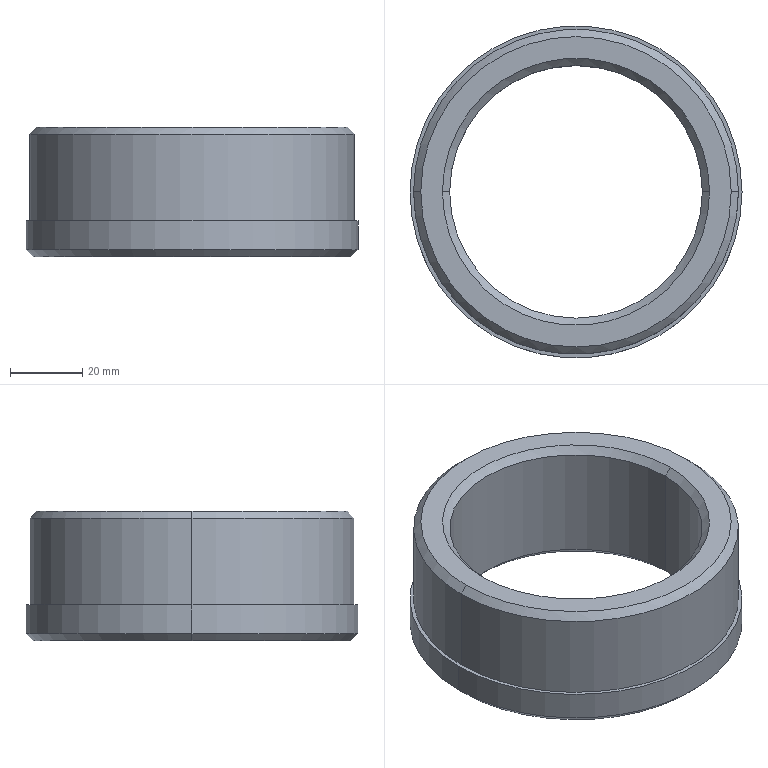Part | SolidWorks | features Chamfer 1, Revolution 1 | 1 solid | 17 faces | box 92 x 92 x 36 mm | volume 91314 mm3 | cone 8 | cylinder 6 | plane 3 | commonest cylinder face diameters 70 x2 90 x2 92 x2
STEP:
#1=CARTESIAN_POINT('',(43.,0.,0.));
#2=VERTEX_POINT('',#1);
#3=CARTESIAN_POINT('',(-43.,0.,0.));
#4=VERTEX_POINT('',#3);
#5=CARTESIAN_POINT('',(0.,0.,0.));
#6=DIRECTION('',(0.,0.,1.));
#7=DIRECTION('',(1.,0.,0.));
#8=AXIS2_PLACEMENT_3D('',#5,#6,#7);
#9=CIRCLE('',#8,43.);
#10=EDGE_CURVE('',#2,#4,#9,.T.);
#11=ORIENTED_EDGE('',*,*,#10,.F.);
#12=CARTESIAN_POINT('',(45.,0.,-2.));
#13=VERTEX_POINT('',#12);
#14=CARTESIAN_POINT('',(43.,0.,0.));
#15=DIRECTION('',(0.7071,0.,-0.7071));
#16=VECTOR('',#15,1000.);
#17=LINE('',#14,#16);
#18=EDGE_CURVE('',#2,#13,#17,.T.);
#19=ORIENTED_EDGE('',*,*,#18,.T.);
#20=CARTESIAN_POINT('',(-45.,0.,-2.));
#21=VERTEX_POINT('',#20);
#22=CARTESIAN_POINT('',(0.,0.,-2.));
#23=DIRECTION('',(0.,0.,-1.));
#24=DIRECTION('',(1.,0.,0.));
#25=AXIS2_PLACEMENT_3D('',#22,#23,#24);
#26=CIRCLE('',#25,45.);
#27=EDGE_CURVE('',#21,#13,#26,.T.);
#28=ORIENTED_EDGE('',*,*,#27,.F.);
#29=CARTESIAN_POINT('',(-43.,0.,0.));
#30=DIRECTION('',(-0.7071,0.,-0.7071));
#31=VECTOR('',#30,1000.);
#32=LINE('',#29,#31);
#33=EDGE_CURVE('',#4,#21,#32,.T.);
#34=ORIENTED_EDGE('',*,*,#33,.F.);
#35=EDGE_LOOP('',(#11,#19,#28,#34));
#36=FACE_OUTER_BOUND('',#35,.T.);
#37=CARTESIAN_POINT('',(0.,0.,0.));
#38=DIRECTION('',(0.,0.,-1.));
#39=DIRECTION('',(-1.,0.,0.));
#40=AXIS2_PLACEMENT_3D('',#37,#38,#39);
#41=CONICAL_SURFACE('',#40,43.,0.7854);
#42=ADVANCED_FACE('',(#36),#41,.T.);
#43=CARTESIAN_POINT('',(-35.,0.,-2.));
#44=VERTEX_POINT('',#43);
#45=CARTESIAN_POINT('',(35.,0.,-2.));
#46=VERTEX_POINT('',#45);
#47=CARTESIAN_POINT('',(0.,0.,-2.));
#48=DIRECTION('',(0.,0.,1.));
#49=DIRECTION('',(1.,0.,0.));
#50=AXIS2_PLACEMENT_3D('',#47,#48,#49);
#51=CIRCLE('',#50,35.);
#52=EDGE_CURVE('',#44,#46,#51,.T.);
#53=ORIENTED_EDGE('',*,*,#52,.F.);
#54=CARTESIAN_POINT('',(-37.,0.,0.));
#55=VERTEX_POINT('',#54);
#56=CARTESIAN_POINT('',(-35.,0.,-2.));
#57=DIRECTION('',(-0.7071,0.,0.7071));
#58=VECTOR('',#57,1000.);
#59=LINE('',#56,#58);
#60=EDGE_CURVE('',#44,#55,#59,.T.);
#61=ORIENTED_EDGE('',*,*,#60,.T.);
#62=CARTESIAN_POINT('',(37.,0.,0.));
#63=VERTEX_POINT('',#62);
#64=CARTESIAN_POINT('',(0.,0.,0.));
#65=DIRECTION('',(0.,0.,-1.));
#66=DIRECTION('',(1.,0.,0.));
#67=AXIS2_PLACEMENT_3D('',#64,#65,#66);
#68=CIRCLE('',#67,37.);
#69=EDGE_CURVE('',#63,#55,#68,.T.);
#70=ORIENTED_EDGE('',*,*,#69,.F.);
#71=CARTESIAN_POINT('',(35.,0.,-2.));
#72=DIRECTION('',(0.7071,0.,0.7071));
#73=VECTOR('',#72,1000.);
#74=LINE('',#71,#73);
#75=EDGE_CURVE('',#46,#63,#74,.T.);
#76=ORIENTED_EDGE('',*,*,#75,.F.);
#77=EDGE_LOOP('',(#53,#61,#70,#76));
#78=FACE_OUTER_BOUND('',#77,.T.);
#79=CARTESIAN_POINT('',(0.,0.,-2.));
#80=DIRECTION('',(0.,0.,1.));
#81=DIRECTION('',(1.,0.,0.));
#82=AXIS2_PLACEMENT_3D('',#79,#80,#81);
#83=CONICAL_SURFACE('',#82,35.,0.7854);
#84=ADVANCED_FACE('',(#78),#83,.F.);
#85=CARTESIAN_POINT('',(-44.,0.,-36.));
#86=VERTEX_POINT('',#85);
#87=CARTESIAN_POINT('',(44.,0.,-36.));
#88=VERTEX_POINT('',#87);
#89=CARTESIAN_POINT('',(0.,0.,-36.));
#90=DIRECTION('',(0.,0.,-1.));
#91=DIRECTION('',(1.,0.,0.));
#92=AXIS2_PLACEMENT_3D('',#89,#90,#91);
#93=CIRCLE('',#92,44.);
#94=EDGE_CURVE('',#86,#88,#93,.T.);
#95=ORIENTED_EDGE('',*,*,#94,.F.);
#96=CARTESIAN_POINT('',(-46.,0.,-34.));
#97=VERTEX_POINT('',#96);
#98=CARTESIAN_POINT('',(-46.,0.,-34.));
#99=DIRECTION('',(-0.7071,0.,0.7071));
#100=VECTOR('',#99,1000.);
#101=LINE('',#98,#100);
#102=EDGE_CURVE('',#86,#97,#101,.T.);
#103=ORIENTED_EDGE('',*,*,#102,.T.);
#104=CARTESIAN_POINT('',(46.,0.,-34.));
#105=VERTEX_POINT('',#104);
#106=CARTESIAN_POINT('',(0.,0.,-34.));
#107=DIRECTION('',(0.,0.,1.));
#108=DIRECTION('',(1.,0.,0.));
#109=AXIS2_PLACEMENT_3D('',#106,#107,#108);
#110=CIRCLE('',#109,46.);
#111=EDGE_CURVE('',#105,#97,#110,.T.);
#112=ORIENTED_EDGE('',*,*,#111,.F.);
#113=CARTESIAN_POINT('',(46.,0.,-34.));
#114=DIRECTION('',(0.7071,0.,0.7071));
#115=VECTOR('',#114,1000.);
#116=LINE('',#113,#115);
#117=EDGE_CURVE('',#88,#105,#116,.T.);
#118=ORIENTED_EDGE('',*,*,#117,.F.);
#119=EDGE_LOOP('',(#95,#103,#112,#118));
#120=FACE_OUTER_BOUND('',#119,.T.);
#121=CARTESIAN_POINT('',(0.,0.,-34.));
#122=DIRECTION('',(0.,0.,1.));
#123=DIRECTION('',(1.,0.,0.));
#124=AXIS2_PLACEMENT_3D('',#121,#122,#123);
#125=CONICAL_SURFACE('',#124,46.,0.7854);
#126=ADVANCED_FACE('',(#120),#125,.T.);
#127=CARTESIAN_POINT('',(35.,0.,-34.));
#128=VERTEX_POINT('',#127);
#129=CARTESIAN_POINT('',(-35.,0.,-34.));
#130=VERTEX_POINT('',#129);
#131=CARTESIAN_POINT('',(0.,0.,-34.));
#132=DIRECTION('',(0.,0.,-1.));
#133=DIRECTION('',(1.,0.,0.));
#134=AXIS2_PLACEMENT_3D('',#131,#132,#133);
#135=CIRCLE('',#134,35.);
#136=EDGE_CURVE('',#128,#130,#135,.T.);
#137=ORIENTED_EDGE('',*,*,#136,.F.);
#138=CARTESIAN_POINT('',(37.,0.,-36.));
#139=VERTEX_POINT('',#138);
#140=CARTESIAN_POINT('',(37.,0.,-36.));
#141=DIRECTION('',(0.7071,0.,-0.7071));
#142=VECTOR('',#141,1000.);
#143=LINE('',#140,#142);
#144=EDGE_CURVE('',#128,#139,#143,.T.);
#145=ORIENTED_EDGE('',*,*,#144,.T.);
#146=CARTESIAN_POINT('',(-37.,0.,-36.));
#147=VERTEX_POINT('',#146);
#148=CARTESIAN_POINT('',(0.,0.,-36.));
#149=DIRECTION('',(0.,0.,1.));
#150=DIRECTION('',(1.,0.,0.));
#151=AXIS2_PLACEMENT_3D('',#148,#149,#150);
#152=CIRCLE('',#151,37.);
#153=EDGE_CURVE('',#147,#139,#152,.T.);
#154=ORIENTED_EDGE('',*,*,#153,.F.);
#155=CARTESIAN_POINT('',(-37.,0.,-36.));
#156=DIRECTION('',(-0.7071,0.,-0.7071));
#157=VECTOR('',#156,1000.);
#158=LINE('',#155,#157);
#159=EDGE_CURVE('',#130,#147,#158,.T.);
#160=ORIENTED_EDGE('',*,*,#159,.F.);
#161=EDGE_LOOP('',(#137,#145,#154,#160));
#162=FACE_OUTER_BOUND('',#161,.T.);
#163=CARTESIAN_POINT('',(0.,0.,-36.));
#164=DIRECTION('',(0.,0.,-1.));
#165=DIRECTION('',(-1.,0.,0.));
#166=AXIS2_PLACEMENT_3D('',#163,#164,#165);
#167=CONICAL_SURFACE('',#166,37.,0.7854);
#168=ADVANCED_FACE('',(#162),#167,.F.);
#169=CARTESIAN_POINT('',(45.,0.,-26.));
#170=VERTEX_POINT('',#169);
#171=CARTESIAN_POINT('',(-45.,0.,-26.));
#172=VERTEX_POINT('',#171);
#173=CARTESIAN_POINT('',(0.,0.,-26.));
#174=DIRECTION('',(0.,0.,1.));
#175=DIRECTION('',(1.,0.,0.));
#176=AXIS2_PLACEMENT_3D('',#173,#174,#175);
#177=CIRCLE('',#176,45.);
#178=EDGE_CURVE('',#170,#172,#177,.T.);
#179=ORIENTED_EDGE('',*,*,#178,.T.);
#180=CARTESIAN_POINT('',(-45.,0.,0.));
#181=DIRECTION('',(0.,0.,1.));
#182=VECTOR('',#181,1000.);
#183=LINE('',#180,#182);
#184=EDGE_CURVE('',#172,#21,#183,.T.);
#185=ORIENTED_EDGE('',*,*,#184,.T.);
#186=ORIENTED_EDGE('',*,*,#27,.T.);
#187=CARTESIAN_POINT('',(45.,0.,0.));
#188=DIRECTION('',(0.,0.,1.));
#189=VECTOR('',#188,1000.);
#190=LINE('',#187,#189);
#191=EDGE_CURVE('',#170,#13,#190,.T.);
#192=ORIENTED_EDGE('',*,*,#191,.F.);
#193=EDGE_LOOP('',(#179,#185,#186,#192));
#194=FACE_OUTER_BOUND('',#193,.T.);
#195=CARTESIAN_POINT('',(0.,0.,0.));
#196=DIRECTION('',(0.,0.,1.));
#197=DIRECTION('',(1.,0.,0.));
#198=AXIS2_PLACEMENT_3D('',#195,#196,#197);
#199=CYLINDRICAL_SURFACE('',#198,45.);
#200=ADVANCED_FACE('',(#194),#199,.T.);
#201=ORIENTED_EDGE('',*,*,#111,.T.);
#202=CARTESIAN_POINT('',(-46.,0.,-26.));
#203=VERTEX_POINT('',#202);
#204=CARTESIAN_POINT('',(-46.,0.,0.));
#205=DIRECTION('',(0.,0.,1.));
#206=VECTOR('',#205,1000.);
#207=LINE('',#204,#206);
#208=EDGE_CURVE('',#97,#203,#207,.T.);
#209=ORIENTED_EDGE('',*,*,#208,.T.);
#210=CARTESIAN_POINT('',(46.,0.,-26.));
#211=VERTEX_POINT('',#210);
#212=CARTESIAN_POINT('',(0.,0.,-26.));
#213=DIRECTION('',(0.,0.,1.));
#214=DIRECTION('',(1.,0.,0.));
#215=AXIS2_PLACEMENT_3D('',#212,#213,#214);
#216=CIRCLE('',#215,46.);
#217=EDGE_CURVE('',#211,#203,#216,.T.);
#218=ORIENTED_EDGE('',*,*,#217,.F.);
#219=CARTESIAN_POINT('',(46.,0.,0.));
#220=DIRECTION('',(0.,0.,1.));
#221=VECTOR('',#220,1000.);
#222=LINE('',#219,#221);
#223=EDGE_CURVE('',#105,#211,#222,.T.);
#224=ORIENTED_EDGE('',*,*,#223,.F.);
#225=EDGE_LOOP('',(#201,#209,#218,#224));
#226=FACE_OUTER_BOUND('',#225,.T.);
#227=CARTESIAN_POINT('',(0.,0.,0.));
#228=DIRECTION('',(0.,0.,1.));
#229=DIRECTION('',(1.,0.,0.));
#230=AXIS2_PLACEMENT_3D('',#227,#228,#229);
#231=CYLINDRICAL_SURFACE('',#230,46.);
#232=ADVANCED_FACE('',(#226),#231,.T.);
#233=ORIENTED_EDGE('',*,*,#136,.T.);
#234=CARTESIAN_POINT('',(-35.,0.,0.));
#235=DIRECTION('',(0.,0.,1.));
#236=VECTOR('',#235,1000.);
#237=LINE('',#234,#236);
#238=EDGE_CURVE('',#130,#44,#237,.T.);
#239=ORIENTED_EDGE('',*,*,#238,.T.);
#240=ORIENTED_EDGE('',*,*,#52,.T.);
#241=CARTESIAN_POINT('',(35.,0.,0.));
#242=DIRECTION('',(0.,0.,1.));
#243=VECTOR('',#242,1000.);
#244=LINE('',#241,#243);
#245=EDGE_CURVE('',#128,#46,#244,.T.);
#246=ORIENTED_EDGE('',*,*,#245,.F.);
#247=EDGE_LOOP('',(#233,#239,#240,#246));
#248=FACE_OUTER_BOUND('',#247,.T.);
#249=CARTESIAN_POINT('',(0.,0.,0.));
#250=DIRECTION('',(0.,0.,1.));
#251=DIRECTION('',(1.,0.,0.));
#252=AXIS2_PLACEMENT_3D('',#249,#250,#251);
#253=CYLINDRICAL_SURFACE('',#252,35.);
#254=ADVANCED_FACE('',(#248),#253,.F.);
#255=ORIENTED_EDGE('',*,*,#69,.T.);
#256=CARTESIAN_POINT('',(0.,0.,0.));
#257=DIRECTION('',(0.,0.,-1.));
#258=DIRECTION('',(1.,0.,0.));
#259=AXIS2_PLACEMENT_3D('',#256,#257,#258);
#260=CIRCLE('',#259,37.);
#261=EDGE_CURVE('',#55,#63,#260,.T.);
#262=ORIENTED_EDGE('',*,*,#261,.T.);
#263=EDGE_LOOP('',(#255,#262));
#264=FACE_BOUND('',#263,.T.);
#265=CARTESIAN_POINT('',(0.,0.,0.));
#266=DIRECTION('',(0.,0.,1.));
#267=DIRECTION('',(1.,0.,0.));
#268=AXIS2_PLACEMENT_3D('',#265,#266,#267);
#269=CIRCLE('',#268,43.);
#270=EDGE_CURVE('',#4,#2,#269,.T.);
#271=ORIENTED_EDGE('',*,*,#270,.T.);
#272=ORIENTED_EDGE('',*,*,#10,.T.);
#273=EDGE_LOOP('',(#271,#272));
#274=FACE_OUTER_BOUND('',#273,.T.);
#275=CARTESIAN_POINT('',(0.,0.,0.));
#276=DIRECTION('',(0.,0.,1.));
#277=DIRECTION('',(1.,0.,0.));
#278=AXIS2_PLACEMENT_3D('',#275,#276,#277);
#279=PLANE('',#278);
#280=ADVANCED_FACE('',(#264,#274),#279,.T.);
#281=ORIENTED_EDGE('',*,*,#238,.F.);
#282=CARTESIAN_POINT('',(0.,0.,-34.));
#283=DIRECTION('',(0.,0.,-1.));
#284=DIRECTION('',(1.,0.,0.));
#285=AXIS2_PLACEMENT_3D('',#282,#283,#284);
#286=CIRCLE('',#285,35.);
#287=EDGE_CURVE('',#130,#128,#286,.T.);
#288=ORIENTED_EDGE('',*,*,#287,.T.);
#289=ORIENTED_EDGE('',*,*,#245,.T.);
#290=CARTESIAN_POINT('',(0.,0.,-2.));
#291=DIRECTION('',(0.,0.,1.));
#292=DIRECTION('',(1.,0.,0.));
#293=AXIS2_PLACEMENT_3D('',#290,#291,#292);
#294=CIRCLE('',#293,35.);
#295=EDGE_CURVE('',#46,#44,#294,.T.);
#296=ORIENTED_EDGE('',*,*,#295,.T.);
#297=EDGE_LOOP('',(#281,#288,#289,#296));
#298=FACE_OUTER_BOUND('',#297,.T.);
#299=CARTESIAN_POINT('',(0.,0.,0.));
#300=DIRECTION('',(0.,0.,1.));
#301=DIRECTION('',(1.,0.,0.));
#302=AXIS2_PLACEMENT_3D('',#299,#300,#301);
#303=CYLINDRICAL_SURFACE('',#302,35.);
#304=ADVANCED_FACE('',(#298),#303,.F.);
#305=ORIENTED_EDGE('',*,*,#153,.T.);
#306=CARTESIAN_POINT('',(0.,0.,-36.));
#307=DIRECTION('',(0.,0.,1.));
#308=DIRECTION('',(1.,0.,0.));
#309=AXIS2_PLACEMENT_3D('',#306,#307,#308);
#310=CIRCLE('',#309,37.);
#311=EDGE_CURVE('',#139,#147,#310,.T.);
#312=ORIENTED_EDGE('',*,*,#311,.T.);
#313=EDGE_LOOP('',(#305,#312));
#314=FACE_BOUND('',#313,.T.);
#315=CARTESIAN_POINT('',(0.,0.,-36.));
#316=DIRECTION('',(0.,0.,-1.));
#317=DIRECTION('',(1.,0.,0.));
#318=AXIS2_PLACEMENT_3D('',#315,#316,#317);
#319=CIRCLE('',#318,44.);
#320=EDGE_CURVE('',#88,#86,#319,.T.);
#321=ORIENTED_EDGE('',*,*,#320,.T.);
#322=ORIENTED_EDGE('',*,*,#94,.T.);
#323=EDGE_LOOP('',(#321,#322));
#324=FACE_OUTER_BOUND('',#323,.T.);
#325=CARTESIAN_POINT('',(0.,0.,-36.));
#326=DIRECTION('',(0.,0.,1.));
#327=DIRECTION('',(1.,0.,0.));
#328=AXIS2_PLACEMENT_3D('',#325,#326,#327);
#329=PLANE('',#328);
#330=ADVANCED_FACE('',(#314,#324),#329,.F.);
#331=ORIENTED_EDGE('',*,*,#208,.F.);
#332=CARTESIAN_POINT('',(0.,0.,-34.));
#333=DIRECTION('',(0.,0.,1.));
#334=DIRECTION('',(1.,0.,0.));
#335=AXIS2_PLACEMENT_3D('',#332,#333,#334);
#336=CIRCLE('',#335,46.);
#337=EDGE_CURVE('',#97,#105,#336,.T.);
#338=ORIENTED_EDGE('',*,*,#337,.T.);
#339=ORIENTED_EDGE('',*,*,#223,.T.);
#340=CARTESIAN_POINT('',(0.,0.,-26.));
#341=DIRECTION('',(0.,0.,1.));
#342=DIRECTION('',(1.,0.,0.));
#343=AXIS2_PLACEMENT_3D('',#340,#341,#342);
#344=CIRCLE('',#343,46.);
#345=EDGE_CURVE('',#203,#211,#344,.T.);
#346=ORIENTED_EDGE('',*,*,#345,.F.);
#347=EDGE_LOOP('',(#331,#338,#339,#346));
#348=FACE_OUTER_BOUND('',#347,.T.);
#349=CARTESIAN_POINT('',(0.,0.,0.));
#350=DIRECTION('',(0.,0.,1.));
#351=DIRECTION('',(1.,0.,0.));
#352=AXIS2_PLACEMENT_3D('',#349,#350,#351);
#353=CYLINDRICAL_SURFACE('',#352,46.);
#354=ADVANCED_FACE('',(#348),#353,.T.);
#355=ORIENTED_EDGE('',*,*,#217,.T.);
#356=ORIENTED_EDGE('',*,*,#345,.T.);
#357=EDGE_LOOP('',(#355,#356));
#358=FACE_OUTER_BOUND('',#357,.T.);
#359=ORIENTED_EDGE('',*,*,#178,.F.);
#360=CARTESIAN_POINT('',(0.,0.,-26.));
#361=DIRECTION('',(0.,0.,1.));
#362=DIRECTION('',(1.,0.,0.));
#363=AXIS2_PLACEMENT_3D('',#360,#361,#362);
#364=CIRCLE('',#363,45.);
#365=EDGE_CURVE('',#172,#170,#364,.T.);
#366=ORIENTED_EDGE('',*,*,#365,.F.);
#367=EDGE_LOOP('',(#359,#366));
#368=FACE_BOUND('',#367,.T.);
#369=CARTESIAN_POINT('',(0.,0.,-26.));
#370=DIRECTION('',(0.,0.,1.));
#371=DIRECTION('',(1.,0.,0.));
#372=AXIS2_PLACEMENT_3D('',#369,#370,#371);
#373=PLANE('',#372);
#374=ADVANCED_FACE('',(#358,#368),#373,.T.);
#375=ORIENTED_EDGE('',*,*,#184,.F.);
#376=ORIENTED_EDGE('',*,*,#365,.T.);
#377=ORIENTED_EDGE('',*,*,#191,.T.);
#378=CARTESIAN_POINT('',(0.,0.,-2.));
#379=DIRECTION('',(0.,0.,-1.));
#380=DIRECTION('',(1.,0.,0.));
#381=AXIS2_PLACEMENT_3D('',#378,#379,#380);
#382=CIRCLE('',#381,45.);
#383=EDGE_CURVE('',#13,#21,#382,.T.);
#384=ORIENTED_EDGE('',*,*,#383,.T.);
#385=EDGE_LOOP('',(#375,#376,#377,#384));
#386=FACE_OUTER_BOUND('',#385,.T.);
#387=CARTESIAN_POINT('',(0.,0.,0.));
#388=DIRECTION('',(0.,0.,1.));
#389=DIRECTION('',(1.,0.,0.));
#390=AXIS2_PLACEMENT_3D('',#387,#388,#389);
#391=CYLINDRICAL_SURFACE('',#390,45.);
#392=ADVANCED_FACE('',(#386),#391,.T.);
#393=ORIENTED_EDGE('',*,*,#144,.F.);
#394=ORIENTED_EDGE('',*,*,#287,.F.);
#395=ORIENTED_EDGE('',*,*,#159,.T.);
#396=ORIENTED_EDGE('',*,*,#311,.F.);
#397=EDGE_LOOP('',(#393,#394,#395,#396));
#398=FACE_OUTER_BOUND('',#397,.T.);
#399=CARTESIAN_POINT('',(0.,0.,-36.));
#400=DIRECTION('',(0.,0.,-1.));
#401=DIRECTION('',(-1.,0.,0.));
#402=AXIS2_PLACEMENT_3D('',#399,#400,#401);
#403=CONICAL_SURFACE('',#402,37.,0.7854);
#404=ADVANCED_FACE('',(#398),#403,.F.);
#405=ORIENTED_EDGE('',*,*,#102,.F.);
#406=ORIENTED_EDGE('',*,*,#320,.F.);
#407=ORIENTED_EDGE('',*,*,#117,.T.);
#408=ORIENTED_EDGE('',*,*,#337,.F.);
#409=EDGE_LOOP('',(#405,#406,#407,#408));
#410=FACE_OUTER_BOUND('',#409,.T.);
#411=CARTESIAN_POINT('',(0.,0.,-34.));
#412=DIRECTION('',(0.,0.,1.));
#413=DIRECTION('',(1.,0.,0.));
#414=AXIS2_PLACEMENT_3D('',#411,#412,#413);
#415=CONICAL_SURFACE('',#414,46.,0.7854);
#416=ADVANCED_FACE('',(#410),#415,.T.);
#417=ORIENTED_EDGE('',*,*,#60,.F.);
#418=ORIENTED_EDGE('',*,*,#295,.F.);
#419=ORIENTED_EDGE('',*,*,#75,.T.);
#420=ORIENTED_EDGE('',*,*,#261,.F.);
#421=EDGE_LOOP('',(#417,#418,#419,#420));
#422=FACE_OUTER_BOUND('',#421,.T.);
#423=CARTESIAN_POINT('',(0.,0.,-2.));
#424=DIRECTION('',(0.,0.,1.));
#425=DIRECTION('',(1.,0.,0.));
#426=AXIS2_PLACEMENT_3D('',#423,#424,#425);
#427=CONICAL_SURFACE('',#426,35.,0.7854);
#428=ADVANCED_FACE('',(#422),#427,.F.);
#429=ORIENTED_EDGE('',*,*,#18,.F.);
#430=ORIENTED_EDGE('',*,*,#270,.F.);
#431=ORIENTED_EDGE('',*,*,#33,.T.);
#432=ORIENTED_EDGE('',*,*,#383,.F.);
#433=EDGE_LOOP('',(#429,#430,#431,#432));
#434=FACE_OUTER_BOUND('',#433,.T.);
#435=CARTESIAN_POINT('',(0.,0.,0.));
#436=DIRECTION('',(0.,0.,-1.));
#437=DIRECTION('',(-1.,0.,0.));
#438=AXIS2_PLACEMENT_3D('',#435,#436,#437);
#439=CONICAL_SURFACE('',#438,43.,0.7854);
#440=ADVANCED_FACE('',(#434),#439,.T.);
#441=CLOSED_SHELL('',(#42,#84,#126,#168,#200,#232,#254,#280,#304,#330,#354,#374,#392,#404,#416,#428,#440));
#442=MANIFOLD_SOLID_BREP('',#441);
#443=CARTESIAN_POINT('',(0.,0.,0.));
#444=DIRECTION('',(0.,0.,1.));
#445=DIRECTION('',(1.,0.,0.));
#446=AXIS2_PLACEMENT_3D('',#443,#444,#445);
#447=(LENGTH_UNIT()NAMED_UNIT(*)SI_UNIT(.MILLI.,.METRE.));
#448=UNCERTAINTY_MEASURE_WITH_UNIT(LENGTH_MEASURE(0.00001),#447,'','');
#449=(NAMED_UNIT(*)PLANE_ANGLE_UNIT()SI_UNIT($,.RADIAN.));
#450=(NAMED_UNIT(*)SI_UNIT($,.STERADIAN.)SOLID_ANGLE_UNIT());
#451=(GEOMETRIC_REPRESENTATION_CONTEXT(3)GLOBAL_UNCERTAINTY_ASSIGNED_CONTEXT((#448))GLOBAL_UNIT_ASSIGNED_CONTEXT((#447,#449,#450))REPRESENTATION_CONTEXT('',''));
#452=ADVANCED_BREP_SHAPE_REPRESENTATION('',(#442,#446),#451);